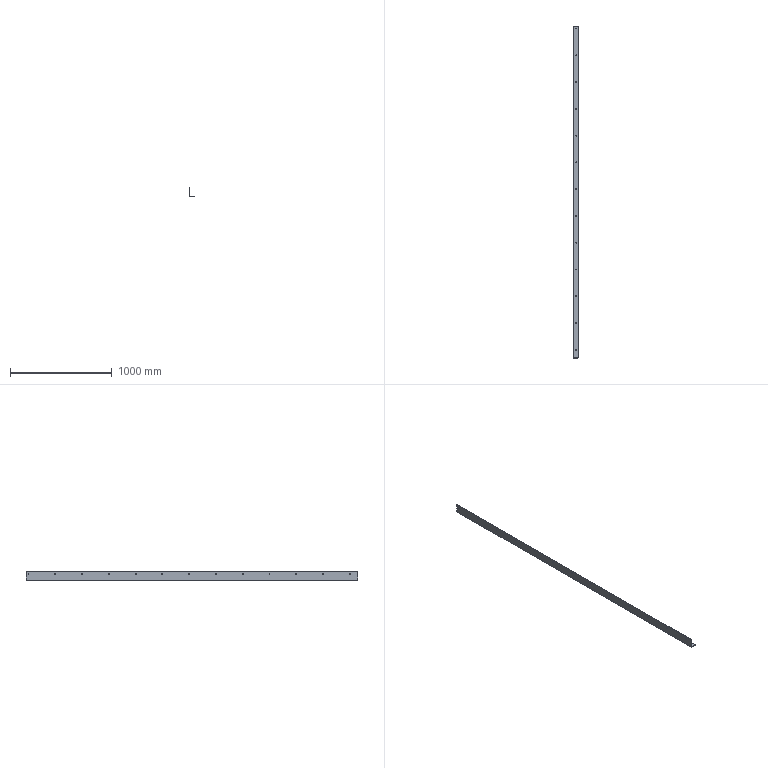Part | STEP file | Assembly TS-S04 | 1 solid | 111 faces | box 55 x 3256 x 90 mm | volume 923542 mm3 | cylinder 72 | plane 39 | commonest cylinder face diameters 8 x65 20 x4 0.4 x1 4.4 x1 10 x1